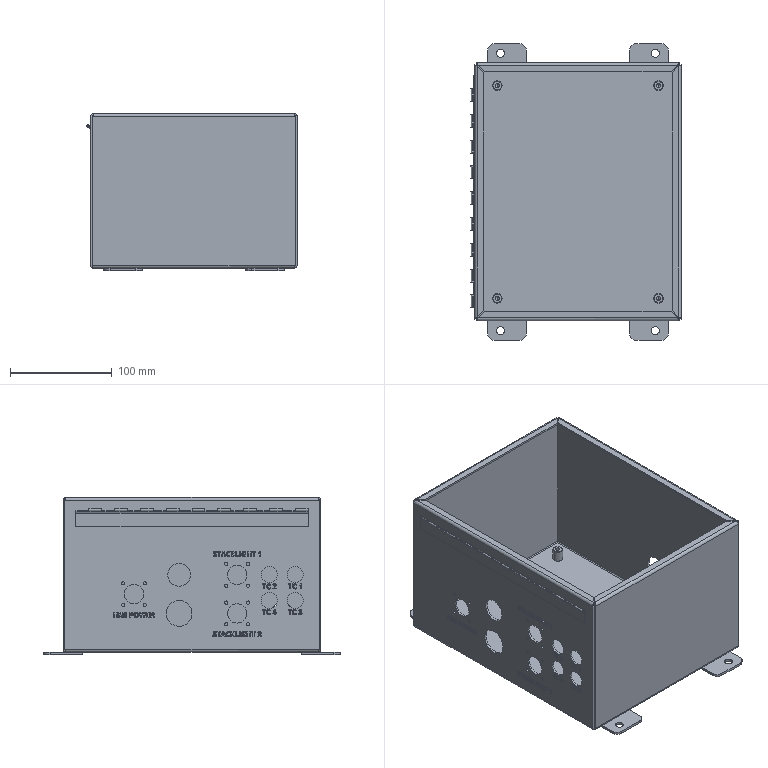Part | SolidWorks | features BaseBody 1 | 1 solid | 1137 faces | box 206.936 x 292.1 x 154.813 mm | volume 362955 mm3 | plane 594 | cylinder 320 | spline 199 | cone 24 | commonest cylinder face diameters 2.54 x27 3.175 x24 12.7 x24 3.337 x12 11.314 x12 2.794 x10